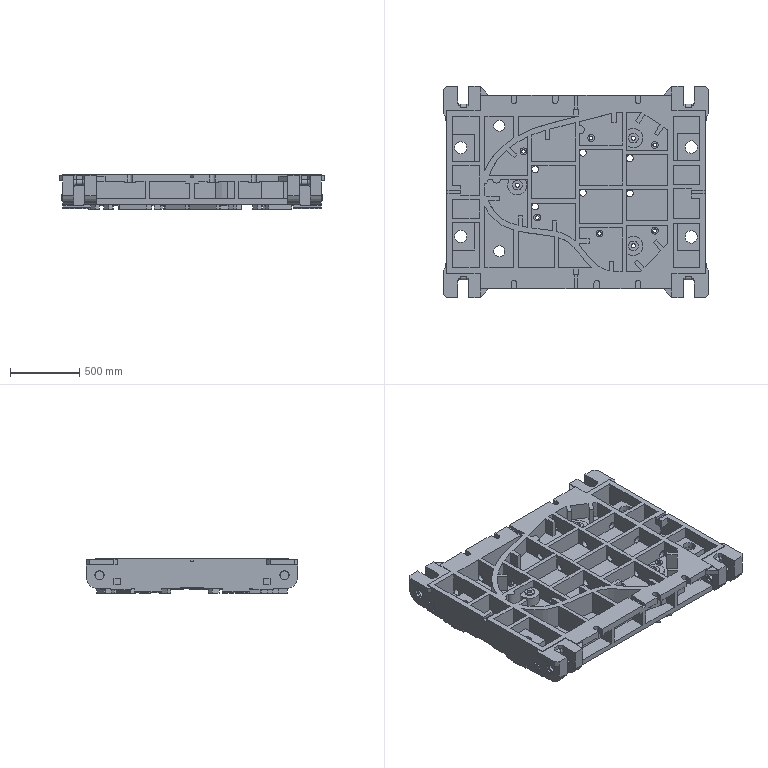Part | NX | features solid 2 | 1 solid | 1183 faces | box 1920 x 1530 x 250 mm | volume 263085210 mm3 | plane 936 | cylinder 202 | spline 37 | torus 8 | commonest cylinder face diameters 68 x48 50 x37 30 x17 60 x16 64 x16 20 x12